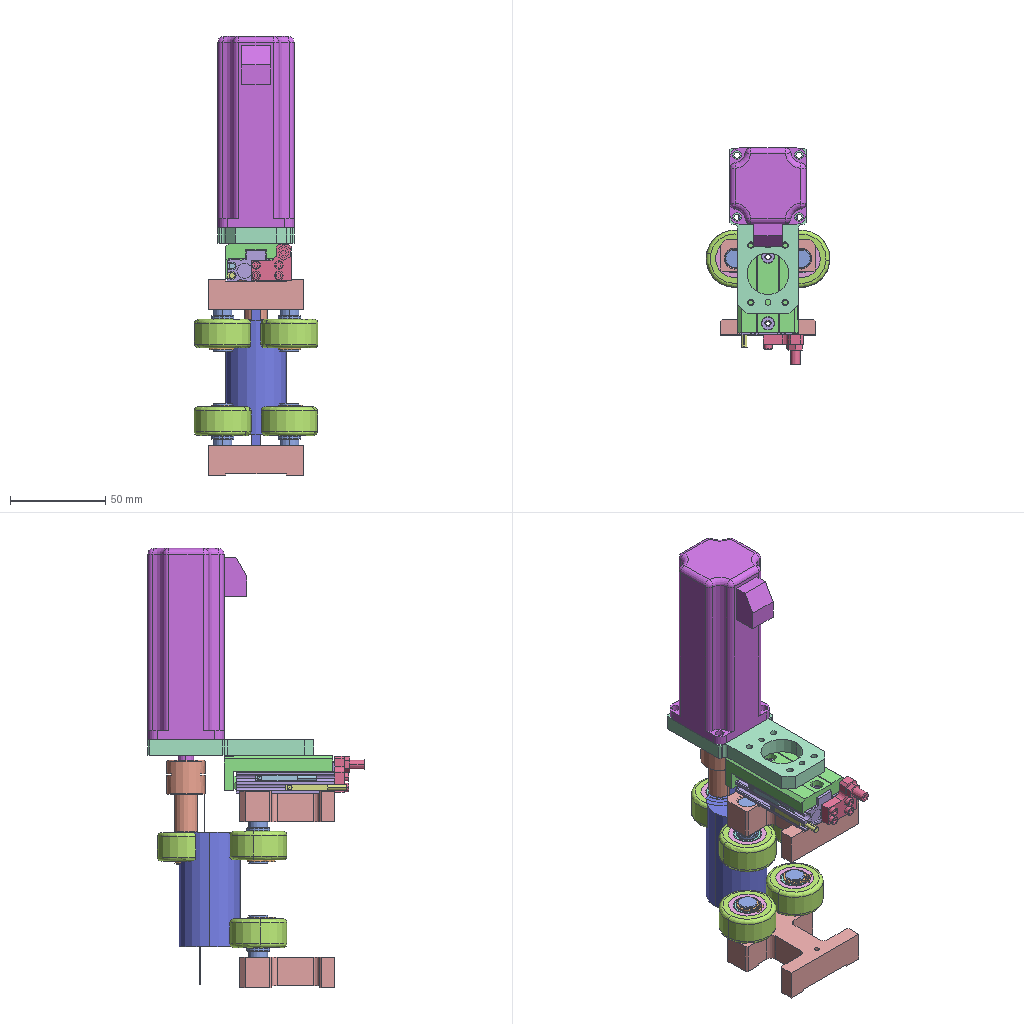Assembly | SolidWorks | 17 different items | 39 placed | box 65 x 113 x 230 mm
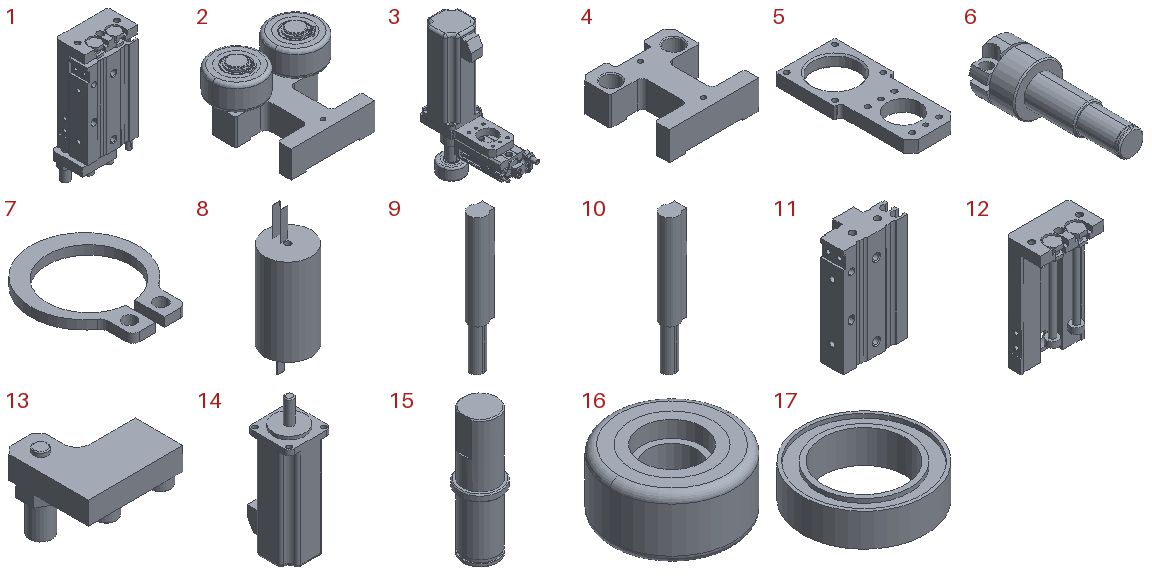Parts list (item | name | quantity | parent item | size | volume | features):
1 | (subassembly) | x1 | in 3 | 34.5 x 20 x 73.5 mm | 32210 mm3 | features AEMSimFeature 1
2 | (subassembly) | x2 | - | 65 x 55 x 38 mm | 43977 mm3 | features AEMSimFeature 1
3 | (subassembly) | x1 | - | 40 x 113.5 x 166.15 mm | 207798 mm3 | features AEMSimFeature 1
4 | - | x2 | in 2 | 50 x 50 x 16 mm | 20170 mm3 | features Chamfer 3, ICE 3, Fillet 2, HoleWzd 2, Extrusion 1
5 | - | x1 | in 3 | 40 x 87 x 8 mm | 15160 mm3 | features Chamfer 2, HoleWzd 2, Extrusion 1, Fillet 1, ICE 1
6 | - | x1 | in 3 | 20 x 55 x 20 mm | 7874 mm3 | features ICE 3, HoleWzd 2, Chamfer 1, Revolution 1
7 | - | x5 | in 2, 3 | 11.91 x 14.373 x 1 mm | 52.893 mm3 | features MoveCopyBody 1, Stock 1
8 | - | x1 | - | 32 x 32 x 100 mm | 47531 mm3 | features ICE 2, Extrusion 1
9 | - | x1 | in 1 | 4.6 x 4 x 32 mm | 394.901 mm3 | features BaseBody 1
10 | - | x1 | in 1 | 4.6 x 4 x 32 mm | 394.901 mm3 | features BaseBody 1
11 | - | x1 | in 1 | 31 x 16 x 51.5 mm | 16230 mm3 | features BaseBody 1
12 | - | x1 | in 1 | 32 x 18.5 x 57 mm | 13333 mm3 | features BaseBody 1
13 | - | x1 | in 1 | 21 x 19 x 16.5 mm | 1857 mm3 | features BaseBody 1
14 | - | x1 | in 3 | 40 x 52 x 126.15 mm | 143595 mm3 | features ICE 5, Fillet 4, Chamfer 2, Extrusion 1, HoleWzd 1
15 | - | x4 | in 2 | 12 x 12 x 37 mm | 2944 mm3 | features ICE 3, Chamfer 1, Extrusion 1, RevCut 1
16 | - | x5 | in 2, 3 | 30 x 30 x 15 mm | 8240 mm3 | features ICE 4, Extrusion 1, Fillet 1
17 | - | x10 | in 2, 3 | 15 x 15 x 4 mm | 333.028 mm3 | features Extrusion 1, ICE 1, MirrorPattern 1
Mates (type | each side: item.copy, entity, surface, feature):
In the top assembly
Coincident | 4.1 face plane Boss-Extrude1 | 4.2 face plane Boss-Extrude1
Coincident | 4.2 face plane Boss-Extrude1 | 4.1 face plane Boss-Extrude1
DistanceDim | 4.1 face plane Boss-Extrude1 | 4.2 face plane Boss-Extrude1
Coincident | 4.2 face plane Boss-Extrude1 | assembly face
Width | 4.2 face | 4.2 face | assembly face | assembly face
DistanceDim | 4.2 face plane Boss-Extrude1 | assembly face
Tangent | 16.1 face cylinder Boss-Extrude2 | 8.1 face cylinder Boss-Extrude1
Tangent | 16.2 face cylinder Boss-Extrude2 | 8.1 face cylinder Boss-Extrude1
Width | 8.1 face plane Boss-Extrude1 | 8.1 face plane Boss-Extrude1 | 4.1 face plane Boss-Extrude1 | 4.2 face plane Boss-Extrude1
Coincident | 4.2 face plane Cut-Extrude2 | 11.1 face plane Input 1
Concentric | 4.2 face cylinder M3 Tapped Hole1 | 11.1 face cylinder Input 1 | 2 times
In subassembly 2
Concentric | 4.3 face cylinder Cut-Extrude1 | 15.1 face cylinder Boss-Extrude1
Coincident | 15.1 face plane Boss-Extrude1 | 4.3 face plane Cut-Extrude2
Parallel | 4.3 face plane Boss-Extrude1 | 15.1 face plane Cut-Extrude1
Concentric | 4.3 face cylinder Cut-Extrude1 | 15.2 face cylinder Boss-Extrude1
Coincident | 4.3 face plane Cut-Extrude2 | 15.2 face plane Boss-Extrude1
Parallel | 4.3 face plane Boss-Extrude1 | 15.2 face plane Cut-Extrude1
Concentric | 15.1 face cylinder Boss-Extrude3 | 16.3 face cylinder Cut-Extrude1
Concentric | 15.1 face cylinder Boss-Extrude3 | 17.1 face cylinder Boss-Extrude1
Concentric | 15.1 face cylinder Boss-Extrude3 | 17.2 face cylinder Boss-Extrude1
Concentric | 15.1 face cylinder Boss-Extrude3 | 7.1 face cylinder (normal) external_is
Coincident | 15.1 face plane Boss-Extrude2 | 17.1 face plane Boss-Extrude1
Coincident | 15.1 face plane Cut-Revolve1 | 7.1 face plane (normal) external_is
Concentric | 15.2 face cylinder Boss-Extrude3 | 17.3 face cylinder Boss-Extrude1
Concentric | 15.2 face cylinder Boss-Extrude3 | 17.4 face cylinder Boss-Extrude1
Concentric | 15.2 face cylinder Boss-Extrude3 | 7.2 face cylinder (normal) external_is
Concentric | 15.2 face cylinder Boss-Extrude3 | 16.4 face cylinder Boss-Extrude2
Coincident | 15.2 face plane Boss-Extrude2 | 17.3 face plane Boss-Extrude1
Coincident | 15.2 face plane Cut-Revolve1 | 7.2 face plane (normal) external_is
Coincident | 16.3 face plane Boss-Extrude1 | 17.1 face plane Boss-Extrude1
Coincident | 16.3 face plane Boss-Extrude1 | 17.2 face plane Boss-Extrude1
Coincident | 16.4 face plane Boss-Extrude1 | 17.3 face plane Boss-Extrude1
Coincident | 16.4 face plane Boss-Extrude1 | 17.4 face plane Boss-Extrude1
In subassembly 3
Coincident | 12.1 face plane Input 1 | 5.1 face plane Boss-Extrude1
Concentric | 12.1 face cylinder Input 1 | 5.1 face cylinder M3 Clearance Hole1 | 2 times
Coincident | 14.1 face plane Boss-Extrude3 | 5.1 face plane Boss-Extrude1
Concentric | 14.1 face cylinder Ø4.5 (4.5) Diameter Hole1 | 5.1 face cylinder M4 Tapped Hole1 | 2 times
Concentric | 16.3 face cylinder Boss-Extrude2 | 14.1 face cylinder Boss-Extrude1
Concentric | 16.3 face cylinder Boss-Extrude2 | 17.2 face cylinder Boss-Extrude1
Concentric | 16.3 face cylinder Boss-Extrude2 | 7.1 face cylinder (normal) external_is
Concentric | 16.3 face cylinder Boss-Extrude2 | 17.1 face cylinder Boss-Extrude1
Concentric | 14.1 face cylinder Boss-Extrude1 | 6.1 face cylinder Revolve1
Coincident | 17.2 face plane Boss-Extrude1 | 6.1 face plane Revolve1
Coincident | 17.2 face plane Boss-Extrude1 | 16.3 face plane Boss-Extrude1
Coincident | 17.1 face plane Boss-Extrude1 | 16.3 face plane Cut-Extrude3
Coincident | 7.1 face plane (normal) external_is | 6.1 face plane Revolve1
DistanceDim | 6.1 face plane Revolve1 | 14.1 face plane Boss-Extrude1
In subassembly 1
Concentric | 11.2 face cylinder Input 1 | 12.2 face cylinder Input 1 | 2 times
LimitDistanceDim | 12.2 face plane Input 1 | 11.2 face plane Input 1
Concentric | 11.2 face cylinder Input 1 | 13.1 face cylinder Input 1 | 2 times
Coincident | 11.2 face plane Input 1 | 13.1 face plane Input 1
DistanceDim | 11.2 face plane Input 1 | 9.1 face plane Input 1
Concentric | 11.2 face cylinder Input 1 | 9.1 face cylinder Input 1
Parallel | 11.2 face plane Input 1 | 9.1 face plane Input 1
DistanceDim | 10.1 face plane Input 1 | 11.2 face plane Input 1
Concentric | 11.2 face cylinder Input 1 | 10.1 face cylinder Input 1
Parallel | 11.2 face plane Input 1 | 10.1 face plane Input 1